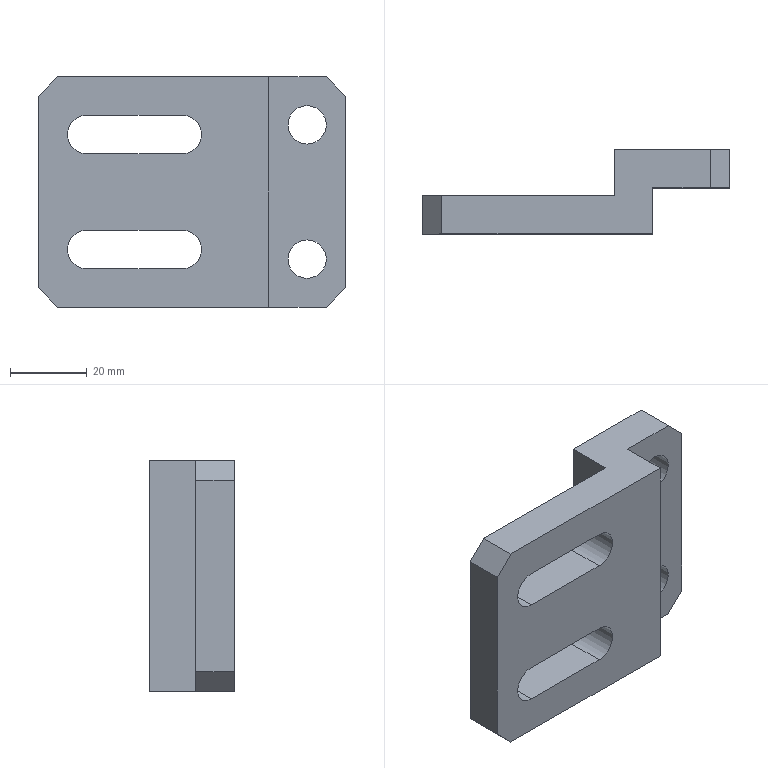Part | SolidWorks | features HoleWzd 2, Chamfer 1, Extrusion 1 | 1 solid | 26 faces | box 80 x 22 x 60 mm | volume 46558 mm3 | plane 18 | cylinder 8 | commonest cylinder face diameters 10 x8
STEP:
#1=CARTESIAN_POINT('',(10.,12.,-22.5));
#2=VERTEX_POINT('',#1);
#3=CARTESIAN_POINT('',(10.,12.,-12.5));
#4=VERTEX_POINT('',#3);
#5=CARTESIAN_POINT('',(10.,12.,-17.5));
#6=DIRECTION('',(0.,1.,0.));
#7=DIRECTION('',(0.,0.,1.));
#8=AXIS2_PLACEMENT_3D('',#5,#6,#7);
#9=CIRCLE('',#8,5.);
#10=EDGE_CURVE('',#2,#4,#9,.T.);
#11=ORIENTED_EDGE('',*,*,#10,.F.);
#12=CARTESIAN_POINT('',(10.,22.,-22.5));
#13=VERTEX_POINT('',#12);
#14=CARTESIAN_POINT('',(10.,22.,-22.5));
#15=DIRECTION('',(0.,1.,0.));
#16=VECTOR('',#15,1000.);
#17=LINE('',#14,#16);
#18=EDGE_CURVE('',#2,#13,#17,.T.);
#19=ORIENTED_EDGE('',*,*,#18,.T.);
#20=CARTESIAN_POINT('',(10.,22.,-12.5));
#21=VERTEX_POINT('',#20);
#22=CARTESIAN_POINT('',(10.,22.,-17.5));
#23=DIRECTION('',(0.,1.,0.));
#24=DIRECTION('',(0.,0.,1.));
#25=AXIS2_PLACEMENT_3D('',#22,#23,#24);
#26=CIRCLE('',#25,5.);
#27=EDGE_CURVE('',#13,#21,#26,.T.);
#28=ORIENTED_EDGE('',*,*,#27,.T.);
#29=CARTESIAN_POINT('',(10.,22.,-12.5));
#30=DIRECTION('',(0.,1.,0.));
#31=VECTOR('',#30,1000.);
#32=LINE('',#29,#31);
#33=EDGE_CURVE('',#4,#21,#32,.T.);
#34=ORIENTED_EDGE('',*,*,#33,.F.);
#35=EDGE_LOOP('',(#11,#19,#28,#34));
#36=FACE_OUTER_BOUND('',#35,.T.);
#37=CARTESIAN_POINT('',(10.,22.,-17.5));
#38=DIRECTION('',(0.,1.,0.));
#39=DIRECTION('',(0.,0.,1.));
#40=AXIS2_PLACEMENT_3D('',#37,#38,#39);
#41=CYLINDRICAL_SURFACE('',#40,5.);
#42=ADVANCED_FACE('',(#36),#41,.F.);
#43=CARTESIAN_POINT('',(10.,12.,12.5));
#44=VERTEX_POINT('',#43);
#45=CARTESIAN_POINT('',(10.,12.,22.5));
#46=VERTEX_POINT('',#45);
#47=CARTESIAN_POINT('',(10.,12.,17.5));
#48=DIRECTION('',(0.,1.,0.));
#49=DIRECTION('',(0.,0.,1.));
#50=AXIS2_PLACEMENT_3D('',#47,#48,#49);
#51=CIRCLE('',#50,5.);
#52=EDGE_CURVE('',#44,#46,#51,.T.);
#53=ORIENTED_EDGE('',*,*,#52,.F.);
#54=CARTESIAN_POINT('',(10.,22.,12.5));
#55=VERTEX_POINT('',#54);
#56=CARTESIAN_POINT('',(10.,22.,12.5));
#57=DIRECTION('',(0.,1.,0.));
#58=VECTOR('',#57,1000.);
#59=LINE('',#56,#58);
#60=EDGE_CURVE('',#44,#55,#59,.T.);
#61=ORIENTED_EDGE('',*,*,#60,.T.);
#62=CARTESIAN_POINT('',(10.,22.,22.5));
#63=VERTEX_POINT('',#62);
#64=CARTESIAN_POINT('',(10.,22.,17.5));
#65=DIRECTION('',(0.,1.,0.));
#66=DIRECTION('',(0.,0.,1.));
#67=AXIS2_PLACEMENT_3D('',#64,#65,#66);
#68=CIRCLE('',#67,5.);
#69=EDGE_CURVE('',#55,#63,#68,.T.);
#70=ORIENTED_EDGE('',*,*,#69,.T.);
#71=CARTESIAN_POINT('',(10.,22.,22.5));
#72=DIRECTION('',(0.,1.,0.));
#73=VECTOR('',#72,1000.);
#74=LINE('',#71,#73);
#75=EDGE_CURVE('',#46,#63,#74,.T.);
#76=ORIENTED_EDGE('',*,*,#75,.F.);
#77=EDGE_LOOP('',(#53,#61,#70,#76));
#78=FACE_OUTER_BOUND('',#77,.T.);
#79=CARTESIAN_POINT('',(10.,22.,17.5));
#80=DIRECTION('',(0.,1.,0.));
#81=DIRECTION('',(0.,0.,1.));
#82=AXIS2_PLACEMENT_3D('',#79,#80,#81);
#83=CYLINDRICAL_SURFACE('',#82,5.);
#84=ADVANCED_FACE('',(#78),#83,.F.);
#85=CARTESIAN_POINT('',(-10.,10.,-30.));
#86=VERTEX_POINT('',#85);
#87=CARTESIAN_POINT('',(-55.,10.,-30.));
#88=VERTEX_POINT('',#87);
#89=CARTESIAN_POINT('',(-10.,10.,-30.));
#90=DIRECTION('',(-1.,0.,0.));
#91=VECTOR('',#90,1000.);
#92=LINE('',#89,#91);
#93=EDGE_CURVE('',#86,#88,#92,.T.);
#94=ORIENTED_EDGE('',*,*,#93,.T.);
#95=CARTESIAN_POINT('',(-60.,10.,-25.));
#96=VERTEX_POINT('',#95);
#97=CARTESIAN_POINT('',(-60.,10.,-25.));
#98=DIRECTION('',(-0.7071,0.,0.7071));
#99=VECTOR('',#98,1000.);
#100=LINE('',#97,#99);
#101=EDGE_CURVE('',#88,#96,#100,.T.);
#102=ORIENTED_EDGE('',*,*,#101,.T.);
#103=CARTESIAN_POINT('',(-60.,10.,25.));
#104=VERTEX_POINT('',#103);
#105=CARTESIAN_POINT('',(-60.,10.,30.));
#106=DIRECTION('',(0.,0.,-1.));
#107=VECTOR('',#106,1000.);
#108=LINE('',#105,#107);
#109=EDGE_CURVE('',#104,#96,#108,.T.);
#110=ORIENTED_EDGE('',*,*,#109,.F.);
#111=CARTESIAN_POINT('',(-55.,10.,30.));
#112=VERTEX_POINT('',#111);
#113=CARTESIAN_POINT('',(-55.,10.,30.));
#114=DIRECTION('',(0.7071,0.,0.7071));
#115=VECTOR('',#114,1000.);
#116=LINE('',#113,#115);
#117=EDGE_CURVE('',#104,#112,#116,.T.);
#118=ORIENTED_EDGE('',*,*,#117,.T.);
#119=CARTESIAN_POINT('',(-10.,10.,30.));
#120=VERTEX_POINT('',#119);
#121=CARTESIAN_POINT('',(-10.,10.,30.));
#122=DIRECTION('',(-1.,0.,0.));
#123=VECTOR('',#122,1000.);
#124=LINE('',#121,#123);
#125=EDGE_CURVE('',#120,#112,#124,.T.);
#126=ORIENTED_EDGE('',*,*,#125,.F.);
#127=CARTESIAN_POINT('',(-10.,10.,30.));
#128=DIRECTION('',(0.,0.,-1.));
#129=VECTOR('',#128,1000.);
#130=LINE('',#127,#129);
#131=EDGE_CURVE('',#120,#86,#130,.T.);
#132=ORIENTED_EDGE('',*,*,#131,.T.);
#133=EDGE_LOOP('',(#94,#102,#110,#118,#126,#132));
#134=FACE_OUTER_BOUND('',#133,.T.);
#135=CARTESIAN_POINT('',(-47.5,10.,10.));
#136=VERTEX_POINT('',#135);
#137=CARTESIAN_POINT('',(-47.5,10.,20.));
#138=VERTEX_POINT('',#137);
#139=CARTESIAN_POINT('',(-47.5,10.,15.));
#140=DIRECTION('',(0.,1.,0.));
#141=DIRECTION('',(0.,0.,1.));
#142=AXIS2_PLACEMENT_3D('',#139,#140,#141);
#143=CIRCLE('',#142,5.);
#144=EDGE_CURVE('',#136,#138,#143,.T.);
#145=ORIENTED_EDGE('',*,*,#144,.F.);
#146=CARTESIAN_POINT('',(-22.5,10.,10.));
#147=VERTEX_POINT('',#146);
#148=CARTESIAN_POINT('',(-47.5,10.,10.));
#149=DIRECTION('',(1.,0.,0.));
#150=VECTOR('',#149,1000.);
#151=LINE('',#148,#150);
#152=EDGE_CURVE('',#136,#147,#151,.T.);
#153=ORIENTED_EDGE('',*,*,#152,.T.);
#154=CARTESIAN_POINT('',(-22.5,10.,20.));
#155=VERTEX_POINT('',#154);
#156=CARTESIAN_POINT('',(-22.5,10.,15.));
#157=DIRECTION('',(0.,1.,0.));
#158=DIRECTION('',(0.,0.,1.));
#159=AXIS2_PLACEMENT_3D('',#156,#157,#158);
#160=CIRCLE('',#159,5.);
#161=EDGE_CURVE('',#155,#147,#160,.T.);
#162=ORIENTED_EDGE('',*,*,#161,.F.);
#163=CARTESIAN_POINT('',(-47.5,10.,20.));
#164=DIRECTION('',(1.,0.,0.));
#165=VECTOR('',#164,1000.);
#166=LINE('',#163,#165);
#167=EDGE_CURVE('',#138,#155,#166,.T.);
#168=ORIENTED_EDGE('',*,*,#167,.F.);
#169=EDGE_LOOP('',(#145,#153,#162,#168));
#170=FACE_BOUND('',#169,.T.);
#171=CARTESIAN_POINT('',(-47.5,10.,-10.));
#172=VERTEX_POINT('',#171);
#173=CARTESIAN_POINT('',(-22.5,10.,-10.));
#174=VERTEX_POINT('',#173);
#175=CARTESIAN_POINT('',(-47.5,10.,-10.));
#176=DIRECTION('',(1.,0.,0.));
#177=VECTOR('',#176,1000.);
#178=LINE('',#175,#177);
#179=EDGE_CURVE('',#172,#174,#178,.T.);
#180=ORIENTED_EDGE('',*,*,#179,.F.);
#181=CARTESIAN_POINT('',(-47.5,10.,-20.));
#182=VERTEX_POINT('',#181);
#183=CARTESIAN_POINT('',(-47.5,10.,-15.));
#184=DIRECTION('',(0.,1.,0.));
#185=DIRECTION('',(0.,0.,1.));
#186=AXIS2_PLACEMENT_3D('',#183,#184,#185);
#187=CIRCLE('',#186,5.);
#188=EDGE_CURVE('',#182,#172,#187,.T.);
#189=ORIENTED_EDGE('',*,*,#188,.F.);
#190=CARTESIAN_POINT('',(-22.5,10.,-20.));
#191=VERTEX_POINT('',#190);
#192=CARTESIAN_POINT('',(-47.5,10.,-20.));
#193=DIRECTION('',(1.,0.,0.));
#194=VECTOR('',#193,1000.);
#195=LINE('',#192,#194);
#196=EDGE_CURVE('',#182,#191,#195,.T.);
#197=ORIENTED_EDGE('',*,*,#196,.T.);
#198=CARTESIAN_POINT('',(-22.5,10.,-15.));
#199=DIRECTION('',(0.,1.,0.));
#200=DIRECTION('',(0.,0.,1.));
#201=AXIS2_PLACEMENT_3D('',#198,#199,#200);
#202=CIRCLE('',#201,5.);
#203=EDGE_CURVE('',#174,#191,#202,.T.);
#204=ORIENTED_EDGE('',*,*,#203,.F.);
#205=EDGE_LOOP('',(#180,#189,#197,#204));
#206=FACE_BOUND('',#205,.T.);
#207=CARTESIAN_POINT('',(-10.,10.,30.));
#208=DIRECTION('',(0.,-1.,0.));
#209=DIRECTION('',(1.,0.,0.));
#210=AXIS2_PLACEMENT_3D('',#207,#208,#209);
#211=PLANE('',#210);
#212=ADVANCED_FACE('',(#134,#170,#206),#211,.F.);
#213=CARTESIAN_POINT('',(-47.5,0.,-10.));
#214=VERTEX_POINT('',#213);
#215=CARTESIAN_POINT('',(-22.5,0.,-10.));
#216=VERTEX_POINT('',#215);
#217=CARTESIAN_POINT('',(-47.5,0.,-10.));
#218=DIRECTION('',(1.,0.,0.));
#219=VECTOR('',#218,1000.);
#220=LINE('',#217,#219);
#221=EDGE_CURVE('',#214,#216,#220,.T.);
#222=ORIENTED_EDGE('',*,*,#221,.T.);
#223=CARTESIAN_POINT('',(-22.5,0.,-20.));
#224=VERTEX_POINT('',#223);
#225=CARTESIAN_POINT('',(-22.5,0.,-15.));
#226=DIRECTION('',(0.,1.,0.));
#227=DIRECTION('',(0.,0.,1.));
#228=AXIS2_PLACEMENT_3D('',#225,#226,#227);
#229=CIRCLE('',#228,5.);
#230=EDGE_CURVE('',#216,#224,#229,.T.);
#231=ORIENTED_EDGE('',*,*,#230,.T.);
#232=CARTESIAN_POINT('',(-47.5,0.,-20.));
#233=VERTEX_POINT('',#232);
#234=CARTESIAN_POINT('',(-47.5,0.,-20.));
#235=DIRECTION('',(1.,0.,0.));
#236=VECTOR('',#235,1000.);
#237=LINE('',#234,#236);
#238=EDGE_CURVE('',#233,#224,#237,.T.);
#239=ORIENTED_EDGE('',*,*,#238,.F.);
#240=CARTESIAN_POINT('',(-47.5,0.,-15.));
#241=DIRECTION('',(0.,1.,0.));
#242=DIRECTION('',(0.,0.,1.));
#243=AXIS2_PLACEMENT_3D('',#240,#241,#242);
#244=CIRCLE('',#243,5.);
#245=EDGE_CURVE('',#233,#214,#244,.T.);
#246=ORIENTED_EDGE('',*,*,#245,.T.);
#247=EDGE_LOOP('',(#222,#231,#239,#246));
#248=FACE_BOUND('',#247,.T.);
#249=CARTESIAN_POINT('',(-60.,0.,25.));
#250=VERTEX_POINT('',#249);
#251=CARTESIAN_POINT('',(-60.,0.,-25.));
#252=VERTEX_POINT('',#251);
#253=CARTESIAN_POINT('',(-60.,0.,30.));
#254=DIRECTION('',(0.,0.,-1.));
#255=VECTOR('',#254,1000.);
#256=LINE('',#253,#255);
#257=EDGE_CURVE('',#250,#252,#256,.T.);
#258=ORIENTED_EDGE('',*,*,#257,.T.);
#259=CARTESIAN_POINT('',(-55.,0.,-30.));
#260=VERTEX_POINT('',#259);
#261=CARTESIAN_POINT('',(-60.,0.,-25.));
#262=DIRECTION('',(0.7071,0.,-0.7071));
#263=VECTOR('',#262,1000.);
#264=LINE('',#261,#263);
#265=EDGE_CURVE('',#252,#260,#264,.T.);
#266=ORIENTED_EDGE('',*,*,#265,.T.);
#267=CARTESIAN_POINT('',(0.,0.,-30.));
#268=VERTEX_POINT('',#267);
#269=CARTESIAN_POINT('',(0.,0.,-30.));
#270=DIRECTION('',(1.,0.,0.));
#271=VECTOR('',#270,1000.);
#272=LINE('',#269,#271);
#273=EDGE_CURVE('',#260,#268,#272,.T.);
#274=ORIENTED_EDGE('',*,*,#273,.T.);
#275=CARTESIAN_POINT('',(0.,0.,30.));
#276=VERTEX_POINT('',#275);
#277=CARTESIAN_POINT('',(0.,0.,30.));
#278=DIRECTION('',(0.,0.,-1.));
#279=VECTOR('',#278,1000.);
#280=LINE('',#277,#279);
#281=EDGE_CURVE('',#276,#268,#280,.T.);
#282=ORIENTED_EDGE('',*,*,#281,.F.);
#283=CARTESIAN_POINT('',(-55.,0.,30.));
#284=VERTEX_POINT('',#283);
#285=CARTESIAN_POINT('',(0.,0.,30.));
#286=DIRECTION('',(1.,0.,0.));
#287=VECTOR('',#286,1000.);
#288=LINE('',#285,#287);
#289=EDGE_CURVE('',#284,#276,#288,.T.);
#290=ORIENTED_EDGE('',*,*,#289,.F.);
#291=CARTESIAN_POINT('',(-55.,0.,30.));
#292=DIRECTION('',(-0.7071,0.,-0.7071));
#293=VECTOR('',#292,1000.);
#294=LINE('',#291,#293);
#295=EDGE_CURVE('',#284,#250,#294,.T.);
#296=ORIENTED_EDGE('',*,*,#295,.T.);
#297=EDGE_LOOP('',(#258,#266,#274,#282,#290,#296));
#298=FACE_OUTER_BOUND('',#297,.T.);
#299=CARTESIAN_POINT('',(-47.5,0.,10.));
#300=VERTEX_POINT('',#299);
#301=CARTESIAN_POINT('',(-22.5,0.,10.));
#302=VERTEX_POINT('',#301);
#303=CARTESIAN_POINT('',(-47.5,0.,10.));
#304=DIRECTION('',(1.,0.,0.));
#305=VECTOR('',#304,1000.);
#306=LINE('',#303,#305);
#307=EDGE_CURVE('',#300,#302,#306,.T.);
#308=ORIENTED_EDGE('',*,*,#307,.F.);
#309=CARTESIAN_POINT('',(-47.5,0.,20.));
#310=VERTEX_POINT('',#309);
#311=CARTESIAN_POINT('',(-47.5,0.,15.));
#312=DIRECTION('',(0.,1.,0.));
#313=DIRECTION('',(0.,0.,1.));
#314=AXIS2_PLACEMENT_3D('',#311,#312,#313);
#315=CIRCLE('',#314,5.);
#316=EDGE_CURVE('',#300,#310,#315,.T.);
#317=ORIENTED_EDGE('',*,*,#316,.T.);
#318=CARTESIAN_POINT('',(-22.5,0.,20.));
#319=VERTEX_POINT('',#318);
#320=CARTESIAN_POINT('',(-47.5,0.,20.));
#321=DIRECTION('',(1.,0.,0.));
#322=VECTOR('',#321,1000.);
#323=LINE('',#320,#322);
#324=EDGE_CURVE('',#310,#319,#323,.T.);
#325=ORIENTED_EDGE('',*,*,#324,.T.);
#326=CARTESIAN_POINT('',(-22.5,0.,15.));
#327=DIRECTION('',(0.,1.,0.));
#328=DIRECTION('',(0.,0.,1.));
#329=AXIS2_PLACEMENT_3D('',#326,#327,#328);
#330=CIRCLE('',#329,5.);
#331=EDGE_CURVE('',#319,#302,#330,.T.);
#332=ORIENTED_EDGE('',*,*,#331,.T.);
#333=EDGE_LOOP('',(#308,#317,#325,#332));
#334=FACE_BOUND('',#333,.T.);
#335=CARTESIAN_POINT('',(0.,0.,30.));
#336=DIRECTION('',(0.,1.,0.));
#337=DIRECTION('',(-1.,0.,0.));
#338=AXIS2_PLACEMENT_3D('',#335,#336,#337);
#339=PLANE('',#338);
#340=ADVANCED_FACE('',(#248,#298,#334),#339,.F.);
#341=CARTESIAN_POINT('',(0.,12.,-30.));
#342=VERTEX_POINT('',#341);
#343=CARTESIAN_POINT('',(0.,0.,-30.));
#344=DIRECTION('',(0.,1.,0.));
#345=VECTOR('',#344,1000.);
#346=LINE('',#343,#345);
#347=EDGE_CURVE('',#268,#342,#346,.T.);
#348=ORIENTED_EDGE('',*,*,#347,.T.);
#349=CARTESIAN_POINT('',(0.,12.,30.));
#350=VERTEX_POINT('',#349);
#351=CARTESIAN_POINT('',(0.,12.,30.));
#352=DIRECTION('',(0.,0.,-1.));
#353=VECTOR('',#352,1000.);
#354=LINE('',#351,#353);
#355=EDGE_CURVE('',#350,#342,#354,.T.);
#356=ORIENTED_EDGE('',*,*,#355,.F.);
#357=CARTESIAN_POINT('',(0.,0.,30.));
#358=DIRECTION('',(0.,1.,0.));
#359=VECTOR('',#358,1000.);
#360=LINE('',#357,#359);
#361=EDGE_CURVE('',#276,#350,#360,.T.);
#362=ORIENTED_EDGE('',*,*,#361,.F.);
#363=ORIENTED_EDGE('',*,*,#281,.T.);
#364=EDGE_LOOP('',(#348,#356,#362,#363));
#365=FACE_OUTER_BOUND('',#364,.T.);
#366=CARTESIAN_POINT('',(0.,0.,30.));
#367=DIRECTION('',(-1.,0.,0.));
#368=DIRECTION('',(0.,0.,1.));
#369=AXIS2_PLACEMENT_3D('',#366,#367,#368);
#370=PLANE('',#369);
#371=ADVANCED_FACE('',(#365),#370,.F.);
#372=CARTESIAN_POINT('',(10.,12.,-17.5));
#373=DIRECTION('',(0.,1.,0.));
#374=DIRECTION('',(0.,0.,1.));
#375=AXIS2_PLACEMENT_3D('',#372,#373,#374);
#376=CIRCLE('',#375,5.);
#377=EDGE_CURVE('',#4,#2,#376,.T.);
#378=ORIENTED_EDGE('',*,*,#377,.T.);
#379=ORIENTED_EDGE('',*,*,#10,.T.);
#380=EDGE_LOOP('',(#378,#379));
#381=FACE_BOUND('',#380,.T.);
#382=CARTESIAN_POINT('',(10.,12.,17.5));
#383=DIRECTION('',(0.,1.,0.));
#384=DIRECTION('',(0.,0.,1.));
#385=AXIS2_PLACEMENT_3D('',#382,#383,#384);
#386=CIRCLE('',#385,5.);
#387=EDGE_CURVE('',#46,#44,#386,.T.);
#388=ORIENTED_EDGE('',*,*,#387,.T.);
#389=ORIENTED_EDGE('',*,*,#52,.T.);
#390=EDGE_LOOP('',(#388,#389));
#391=FACE_BOUND('',#390,.T.);
#392=CARTESIAN_POINT('',(15.,12.,-30.));
#393=VERTEX_POINT('',#392);
#394=CARTESIAN_POINT('',(0.,12.,-30.));
#395=DIRECTION('',(1.,0.,0.));
#396=VECTOR('',#395,1000.);
#397=LINE('',#394,#396);
#398=EDGE_CURVE('',#342,#393,#397,.T.);
#399=ORIENTED_EDGE('',*,*,#398,.T.);
#400=CARTESIAN_POINT('',(20.,12.,-25.));
#401=VERTEX_POINT('',#400);
#402=CARTESIAN_POINT('',(20.,12.,-25.));
#403=DIRECTION('',(0.7071,0.,0.7071));
#404=VECTOR('',#403,1000.);
#405=LINE('',#402,#404);
#406=EDGE_CURVE('',#393,#401,#405,.T.);
#407=ORIENTED_EDGE('',*,*,#406,.T.);
#408=CARTESIAN_POINT('',(20.,12.,25.));
#409=VERTEX_POINT('',#408);
#410=CARTESIAN_POINT('',(20.,12.,30.));
#411=DIRECTION('',(0.,0.,-1.));
#412=VECTOR('',#411,1000.);
#413=LINE('',#410,#412);
#414=EDGE_CURVE('',#409,#401,#413,.T.);
#415=ORIENTED_EDGE('',*,*,#414,.F.);
#416=CARTESIAN_POINT('',(15.,12.,30.));
#417=VERTEX_POINT('',#416);
#418=CARTESIAN_POINT('',(15.,12.,30.));
#419=DIRECTION('',(-0.7071,0.,0.7071));
#420=VECTOR('',#419,1000.);
#421=LINE('',#418,#420);
#422=EDGE_CURVE('',#409,#417,#421,.T.);
#423=ORIENTED_EDGE('',*,*,#422,.T.);
#424=CARTESIAN_POINT('',(0.,12.,30.));
#425=DIRECTION('',(1.,0.,0.));
#426=VECTOR('',#425,1000.);
#427=LINE('',#424,#426);
#428=EDGE_CURVE('',#350,#417,#427,.T.);
#429=ORIENTED_EDGE('',*,*,#428,.F.);
#430=ORIENTED_EDGE('',*,*,#355,.T.);
#431=EDGE_LOOP('',(#399,#407,#415,#423,#429,#430));
#432=FACE_OUTER_BOUND('',#431,.T.);
#433=CARTESIAN_POINT('',(0.,12.,30.));
#434=DIRECTION('',(0.,1.,0.));
#435=DIRECTION('',(0.,0.,1.));
#436=AXIS2_PLACEMENT_3D('',#433,#434,#435);
#437=PLANE('',#436);
#438=ADVANCED_FACE('',(#381,#391,#432),#437,.F.);
#439=ORIENTED_EDGE('',*,*,#414,.T.);
#440=CARTESIAN_POINT('',(20.,22.,-25.));
#441=VERTEX_POINT('',#440);
#442=CARTESIAN_POINT('',(20.,22.,-25.));
#443=DIRECTION('',(0.,1.,0.));
#444=VECTOR('',#443,1000.);
#445=LINE('',#442,#444);
#446=EDGE_CURVE('',#401,#441,#445,.T.);
#447=ORIENTED_EDGE('',*,*,#446,.T.);
#448=CARTESIAN_POINT('',(20.,22.,25.));
#449=VERTEX_POINT('',#448);
#450=CARTESIAN_POINT('',(20.,22.,30.));
#451=DIRECTION('',(0.,0.,-1.));
#452=VECTOR('',#451,1000.);
#453=LINE('',#450,#452);
#454=EDGE_CURVE('',#449,#441,#453,.T.);
#455=ORIENTED_EDGE('',*,*,#454,.F.);
#456=CARTESIAN_POINT('',(20.,12.,25.));
#457=DIRECTION('',(0.,-1.,0.));
#458=VECTOR('',#457,1000.);
#459=LINE('',#456,#458);
#460=EDGE_CURVE('',#449,#409,#459,.T.);
#461=ORIENTED_EDGE('',*,*,#460,.T.);
#462=EDGE_LOOP('',(#439,#447,#455,#461));
#463=FACE_OUTER_BOUND('',#462,.T.);
#464=CARTESIAN_POINT('',(20.,22.,30.));
#465=DIRECTION('',(-1.,0.,0.));
#466=DIRECTION('',(0.,0.,1.));
#467=AXIS2_PLACEMENT_3D('',#464,#465,#466);
#468=PLANE('',#467);
#469=ADVANCED_FACE('',(#463),#468,.F.);
#470=CARTESIAN_POINT('',(10.,22.,-17.5));
#471=DIRECTION('',(0.,1.,0.));
#472=DIRECTION('',(0.,0.,1.));
#473=AXIS2_PLACEMENT_3D('',#470,#471,#472);
#474=CIRCLE('',#473,5.);
#475=EDGE_CURVE('',#21,#13,#474,.T.);
#476=ORIENTED_EDGE('',*,*,#475,.F.);
#477=ORIENTED_EDGE('',*,*,#27,.F.);
#478=EDGE_LOOP('',(#476,#477));
#479=FACE_BOUND('',#478,.T.);
#480=CARTESIAN_POINT('',(10.,22.,17.5));
#481=DIRECTION('',(0.,1.,0.));
#482=DIRECTION('',(0.,0.,1.));
#483=AXIS2_PLACEMENT_3D('',#480,#481,#482);
#484=CIRCLE('',#483,5.);
#485=EDGE_CURVE('',#63,#55,#484,.T.);
#486=ORIENTED_EDGE('',*,*,#485,.F.);
#487=ORIENTED_EDGE('',*,*,#69,.F.);
#488=EDGE_LOOP('',(#486,#487));
#489=FACE_BOUND('',#488,.T.);
#490=ORIENTED_EDGE('',*,*,#454,.T.);
#491=CARTESIAN_POINT('',(15.,22.,-30.));
#492=VERTEX_POINT('',#491);
#493=CARTESIAN_POINT('',(20.,22.,-25.));
#494=DIRECTION('',(-0.7071,0.,-0.7071));
#495=VECTOR('',#494,1000.);
#496=LINE('',#493,#495);
#497=EDGE_CURVE('',#441,#492,#496,.T.);
#498=ORIENTED_EDGE('',*,*,#497,.T.);
#499=CARTESIAN_POINT('',(-10.,22.,-30.));
#500=VERTEX_POINT('',#499);
#501=CARTESIAN_POINT('',(-10.,22.,-30.));
#502=DIRECTION('',(-1.,0.,0.));
#503=VECTOR('',#502,1000.);
#504=LINE('',#501,#503);
#505=EDGE_CURVE('',#492,#500,#504,.T.);
#506=ORIENTED_EDGE('',*,*,#505,.T.);
#507=CARTESIAN_POINT('',(-10.,22.,30.));
#508=VERTEX_POINT('',#507);
#509=CARTESIAN_POINT('',(-10.,22.,30.));
#510=DIRECTION('',(0.,0.,-1.));
#511=VECTOR('',#510,1000.);
#512=LINE('',#509,#511);
#513=EDGE_CURVE('',#508,#500,#512,.T.);
#514=ORIENTED_EDGE('',*,*,#513,.F.);
#515=CARTESIAN_POINT('',(15.,22.,30.));
#516=VERTEX_POINT('',#515);
#517=CARTESIAN_POINT('',(-10.,22.,30.));
#518=DIRECTION('',(-1.,0.,0.));
#519=VECTOR('',#518,1000.);
#520=LINE('',#517,#519);
#521=EDGE_CURVE('',#516,#508,#520,.T.);
#522=ORIENTED_EDGE('',*,*,#521,.F.);
#523=CARTESIAN_POINT('',(15.,22.,30.));
#524=DIRECTION('',(0.7071,0.,-0.7071));
#525=VECTOR('',#524,1000.);
#526=LINE('',#523,#525);
#527=EDGE_CURVE('',#516,#449,#526,.T.);
#528=ORIENTED_EDGE('',*,*,#527,.T.);
#529=EDGE_LOOP('',(#490,#498,#506,#514,#522,#528));
#530=FACE_OUTER_BOUND('',#529,.T.);
#531=CARTESIAN_POINT('',(-10.,22.,30.));
#532=DIRECTION('',(0.,-1.,0.));
#533=DIRECTION('',(0.,0.,-1.));
#534=AXIS2_PLACEMENT_3D('',#531,#532,#533);
#535=PLANE('',#534);
#536=ADVANCED_FACE('',(#479,#489,#530),#535,.F.);
#537=CARTESIAN_POINT('',(-10.,10.,-30.));
#538=DIRECTION('',(0.,-1.,0.));
#539=VECTOR('',#538,1000.);
#540=LINE('',#537,#539);
#541=EDGE_CURVE('',#500,#86,#540,.T.);
#542=ORIENTED_EDGE('',*,*,#541,.T.);
#543=ORIENTED_EDGE('',*,*,#131,.F.);
#544=CARTESIAN_POINT('',(-10.,10.,30.));
#545=DIRECTION('',(0.,-1.,0.));
#546=VECTOR('',#545,1000.);
#547=LINE('',#544,#546);
#548=EDGE_CURVE('',#508,#120,#547,.T.);
#549=ORIENTED_EDGE('',*,*,#548,.F.);
#550=ORIENTED_EDGE('',*,*,#513,.T.);
#551=EDGE_LOOP('',(#542,#543,#549,#550));
#552=FACE_OUTER_BOUND('',#551,.T.);
#553=CARTESIAN_POINT('',(-10.,10.,30.));
#554=DIRECTION('',(1.,0.,0.));
#555=DIRECTION('',(0.,0.,-1.));
#556=AXIS2_PLACEMENT_3D('',#553,#554,#555);
#557=PLANE('',#556);
#558=ADVANCED_FACE('',(#552),#557,.F.);
#559=ORIENTED_EDGE('',*,*,#109,.T.);
#560=CARTESIAN_POINT('',(-60.,10.,-25.));
#561=DIRECTION('',(0.,-1.,0.));
#562=VECTOR('',#561,1000.);
#563=LINE('',#560,#562);
#564=EDGE_CURVE('',#96,#252,#563,.T.);
#565=ORIENTED_EDGE('',*,*,#564,.T.);
#566=ORIENTED_EDGE('',*,*,#257,.F.);
#567=CARTESIAN_POINT('',(-60.,10.,25.));
#568=DIRECTION('',(0.,1.,0.));
#569=VECTOR('',#568,1000.);
#570=LINE('',#567,#569);
#571=EDGE_CURVE('',#250,#104,#570,.T.);
#572=ORIENTED_EDGE('',*,*,#571,.T.);
#573=EDGE_LOOP('',(#559,#565,#566,#572));
#574=FACE_OUTER_BOUND('',#573,.T.);
#575=CARTESIAN_POINT('',(-60.,10.,30.));
#576=DIRECTION('',(1.,0.,0.));
#577=DIRECTION('',(0.,0.,-1.));
#578=AXIS2_PLACEMENT_3D('',#575,#576,#577);
#579=PLANE('',#578);
#580=ADVANCED_FACE('',(#574),#579,.F.);
#581=ORIENTED_EDGE('',*,*,#125,.T.);
#582=CARTESIAN_POINT('',(-55.,0.,30.));
#583=DIRECTION('',(0.,-1.,0.));
#584=VECTOR('',#583,1000.);
#585=LINE('',#582,#584);
#586=EDGE_CURVE('',#112,#284,#585,.T.);
#587=ORIENTED_EDGE('',*,*,#586,.T.);
#588=ORIENTED_EDGE('',*,*,#289,.T.);
#589=ORIENTED_EDGE('',*,*,#361,.T.);
#590=ORIENTED_EDGE('',*,*,#428,.T.);
#591=CARTESIAN_POINT('',(15.,22.,30.));
#592=DIRECTION('',(0.,1.,0.));
#593=VECTOR('',#592,1000.);
#594=LINE('',#591,#593);
#595=EDGE_CURVE('',#417,#516,#594,.T.);
#596=ORIENTED_EDGE('',*,*,#595,.T.);
#597=ORIENTED_EDGE('',*,*,#521,.T.);
#598=ORIENTED_EDGE('',*,*,#548,.T.);
#599=EDGE_LOOP('',(#581,#587,#588,#589,#590,#596,#597,#598));
#600=FACE_OUTER_BOUND('',#599,.T.);
#601=CARTESIAN_POINT('',(0.,0.,30.));
#602=DIRECTION('',(0.,0.,1.));
#603=DIRECTION('',(1.,0.,0.));
#604=AXIS2_PLACEMENT_3D('',#601,#602,#603);
#605=PLANE('',#604);
#606=ADVANCED_FACE('',(#600),#605,.T.);
#607=ORIENTED_EDGE('',*,*,#273,.F.);
#608=CARTESIAN_POINT('',(-55.,0.,-30.));
#609=DIRECTION('',(0.,1.,0.));
#610=VECTOR('',#609,1000.);
#611=LINE('',#608,#610);
#612=EDGE_CURVE('',#260,#88,#611,.T.);
#613=ORIENTED_EDGE('',*,*,#612,.T.);
#614=ORIENTED_EDGE('',*,*,#93,.F.);
#615=ORIENTED_EDGE('',*,*,#541,.F.);
#616=ORIENTED_EDGE('',*,*,#505,.F.);
#617=CARTESIAN_POINT('',(15.,0.,-30.));
#618=DIRECTION('',(0.,-1.,0.));
#619=VECTOR('',#618,1000.);
#620=LINE('',#617,#619);
#621=EDGE_CURVE('',#492,#393,#620,.T.);
#622=ORIENTED_EDGE('',*,*,#621,.T.);
#623=ORIENTED_EDGE('',*,*,#398,.F.);
#624=ORIENTED_EDGE('',*,*,#347,.F.);
#625=EDGE_LOOP('',(#607,#613,#614,#615,#616,#622,#623,#624));
#626=FACE_OUTER_BOUND('',#625,.T.);
#627=CARTESIAN_POINT('',(0.,0.,-30.));
#628=DIRECTION('',(0.,0.,1.));
#629=DIRECTION('',(1.,0.,0.));
#630=AXIS2_PLACEMENT_3D('',#627,#628,#629);
#631=PLANE('',#630);
#632=ADVANCED_FACE('',(#626),#631,.F.);
#633=ORIENTED_EDGE('',*,*,#60,.F.);
#634=ORIENTED_EDGE('',*,*,#387,.F.);
#635=ORIENTED_EDGE('',*,*,#75,.T.);
#636=ORIENTED_EDGE('',*,*,#485,.T.);
#637=EDGE_LOOP('',(#633,#634,#635,#636));
#638=FACE_OUTER_BOUND('',#637,.T.);
#639=CARTESIAN_POINT('',(10.,22.,17.5));
#640=DIRECTION('',(0.,1.,0.));
#641=DIRECTION('',(0.,0.,1.));
#642=AXIS2_PLACEMENT_3D('',#639,#640,#641);
#643=CYLINDRICAL_SURFACE('',#642,5.);
#644=ADVANCED_FACE('',(#638),#643,.F.);
#645=ORIENTED_EDGE('',*,*,#18,.F.);
#646=ORIENTED_EDGE('',*,*,#377,.F.);
#647=ORIENTED_EDGE('',*,*,#33,.T.);
#648=ORIENTED_EDGE('',*,*,#475,.T.);
#649=EDGE_LOOP('',(#645,#646,#647,#648));
#650=FACE_OUTER_BOUND('',#649,.T.);
#651=CARTESIAN_POINT('',(10.,22.,-17.5));
#652=DIRECTION('',(0.,1.,0.));
#653=DIRECTION('',(0.,0.,1.));
#654=AXIS2_PLACEMENT_3D('',#651,#652,#653);
#655=CYLINDRICAL_SURFACE('',#654,5.);
#656=ADVANCED_FACE('',(#650),#655,.F.);
#657=ORIENTED_EDGE('',*,*,#331,.F.);
#658=CARTESIAN_POINT('',(-22.5,10.,20.));
#659=DIRECTION('',(0.,-1.,0.));
#660=VECTOR('',#659,1000.);
#661=LINE('',#658,#660);
#662=EDGE_CURVE('',#155,#319,#661,.T.);
#663=ORIENTED_EDGE('',*,*,#662,.F.);
#664=ORIENTED_EDGE('',*,*,#161,.T.);
#665=CARTESIAN_POINT('',(-22.5,10.,10.));
#666=DIRECTION('',(0.,1.,0.));
#667=VECTOR('',#666,1000.);
#668=LINE('',#665,#667);
#669=EDGE_CURVE('',#302,#147,#668,.T.);
#670=ORIENTED_EDGE('',*,*,#669,.F.);
#671=EDGE_LOOP('',(#657,#663,#664,#670));
#672=FACE_OUTER_BOUND('',#671,.T.);
#673=CARTESIAN_POINT('',(-22.5,10.,15.));
#674=DIRECTION('',(0.,1.,0.));
#675=DIRECTION('',(0.,0.,1.));
#676=AXIS2_PLACEMENT_3D('',#673,#674,#675);
#677=CYLINDRICAL_SURFACE('',#676,5.);
#678=ADVANCED_FACE('',(#672),#677,.F.);
#679=ORIENTED_EDGE('',*,*,#144,.T.);
#680=CARTESIAN_POINT('',(-47.5,10.,20.));
#681=DIRECTION('',(0.,1.,0.));
#682=VECTOR('',#681,1000.);
#683=LINE('',#680,#682);
#684=EDGE_CURVE('',#310,#138,#683,.T.);
#685=ORIENTED_EDGE('',*,*,#684,.F.);
#686=ORIENTED_EDGE('',*,*,#316,.F.);
#687=CARTESIAN_POINT('',(-47.5,10.,10.));
#688=DIRECTION('',(0.,-1.,0.));
#689=VECTOR('',#688,1000.);
#690=LINE('',#687,#689);
#691=EDGE_CURVE('',#136,#300,#690,.T.);
#692=ORIENTED_EDGE('',*,*,#691,.F.);
#693=EDGE_LOOP('',(#679,#685,#686,#692));
#694=FACE_OUTER_BOUND('',#693,.T.);
#695=CARTESIAN_POINT('',(-47.5,10.,15.));
#696=DIRECTION('',(0.,1.,0.));
#697=DIRECTION('',(0.,0.,1.));
#698=AXIS2_PLACEMENT_3D('',#695,#696,#697);
#699=CYLINDRICAL_SURFACE('',#698,5.);
#700=ADVANCED_FACE('',(#694),#699,.F.);
#701=ORIENTED_EDGE('',*,*,#669,.T.);
#702=ORIENTED_EDGE('',*,*,#152,.F.);
#703=ORIENTED_EDGE('',*,*,#691,.T.);
#704=ORIENTED_EDGE('',*,*,#307,.T.);
#705=EDGE_LOOP('',(#701,#702,#703,#704));
#706=FACE_OUTER_BOUND('',#705,.T.);
#707=CARTESIAN_POINT('',(-47.5,10.,10.));
#708=DIRECTION('',(0.,0.,-1.));
#709=DIRECTION('',(-1.,0.,0.));
#710=AXIS2_PLACEMENT_3D('',#707,#708,#709);
#711=PLANE('',#710);
#712=ADVANCED_FACE('',(#706),#711,.F.);
#713=ORIENTED_EDGE('',*,*,#662,.T.);
#714=ORIENTED_EDGE('',*,*,#324,.F.);
#715=ORIENTED_EDGE('',*,*,#684,.T.);
#716=ORIENTED_EDGE('',*,*,#167,.T.);
#717=EDGE_LOOP('',(#713,#714,#715,#716));
#718=FACE_OUTER_BOUND('',#717,.T.);
#719=CARTESIAN_POINT('',(-47.5,10.,20.));
#720=DIRECTION('',(0.,0.,1.));
#721=DIRECTION('',(1.,0.,0.));
#722=AXIS2_PLACEMENT_3D('',#719,#720,#721);
#723=PLANE('',#722);
#724=ADVANCED_FACE('',(#718),#723,.F.);
#725=ORIENTED_EDGE('',*,*,#230,.F.);
#726=CARTESIAN_POINT('',(-22.5,10.,-10.));
#727=DIRECTION('',(0.,-1.,0.));
#728=VECTOR('',#727,1000.);
#729=LINE('',#726,#728);
#730=EDGE_CURVE('',#174,#216,#729,.T.);
#731=ORIENTED_EDGE('',*,*,#730,.F.);
#732=ORIENTED_EDGE('',*,*,#203,.T.);
#733=CARTESIAN_POINT('',(-22.5,10.,-20.));
#734=DIRECTION('',(0.,1.,0.));
#735=VECTOR('',#734,1000.);
#736=LINE('',#733,#735);
#737=EDGE_CURVE('',#224,#191,#736,.T.);
#738=ORIENTED_EDGE('',*,*,#737,.F.);
#739=EDGE_LOOP('',(#725,#731,#732,#738));
#740=FACE_OUTER_BOUND('',#739,.T.);
#741=CARTESIAN_POINT('',(-22.5,10.,-15.));
#742=DIRECTION('',(0.,1.,0.));
#743=DIRECTION('',(0.,0.,1.));
#744=AXIS2_PLACEMENT_3D('',#741,#742,#743);
#745=CYLINDRICAL_SURFACE('',#744,5.);
#746=ADVANCED_FACE('',(#740),#745,.F.);
#747=ORIENTED_EDGE('',*,*,#188,.T.);
#748=CARTESIAN_POINT('',(-47.5,10.,-10.));
#749=DIRECTION('',(0.,1.,0.));
#750=VECTOR('',#749,1000.);
#751=LINE('',#748,#750);
#752=EDGE_CURVE('',#214,#172,#751,.T.);
#753=ORIENTED_EDGE('',*,*,#752,.F.);
#754=ORIENTED_EDGE('',*,*,#245,.F.);
#755=CARTESIAN_POINT('',(-47.5,10.,-20.));
#756=DIRECTION('',(0.,-1.,0.));
#757=VECTOR('',#756,1000.);
#758=LINE('',#755,#757);
#759=EDGE_CURVE('',#182,#233,#758,.T.);
#760=ORIENTED_EDGE('',*,*,#759,.F.);
#761=EDGE_LOOP('',(#747,#753,#754,#760));
#762=FACE_OUTER_BOUND('',#761,.T.);
#763=CARTESIAN_POINT('',(-47.5,10.,-15.));
#764=DIRECTION('',(0.,1.,0.));
#765=DIRECTION('',(0.,0.,1.));
#766=AXIS2_PLACEMENT_3D('',#763,#764,#765);
#767=CYLINDRICAL_SURFACE('',#766,5.);
#768=ADVANCED_FACE('',(#762),#767,.F.);
#769=ORIENTED_EDGE('',*,*,#737,.T.);
#770=ORIENTED_EDGE('',*,*,#196,.F.);
#771=ORIENTED_EDGE('',*,*,#759,.T.);
#772=ORIENTED_EDGE('',*,*,#238,.T.);
#773=EDGE_LOOP('',(#769,#770,#771,#772));
#774=FACE_OUTER_BOUND('',#773,.T.);
#775=CARTESIAN_POINT('',(-47.5,10.,-20.));
#776=DIRECTION('',(0.,0.,-1.));
#777=DIRECTION('',(-1.,0.,0.));
#778=AXIS2_PLACEMENT_3D('',#775,#776,#777);
#779=PLANE('',#778);
#780=ADVANCED_FACE('',(#774),#779,.F.);
#781=ORIENTED_EDGE('',*,*,#730,.T.);
#782=ORIENTED_EDGE('',*,*,#221,.F.);
#783=ORIENTED_EDGE('',*,*,#752,.T.);
#784=ORIENTED_EDGE('',*,*,#179,.T.);
#785=EDGE_LOOP('',(#781,#782,#783,#784));
#786=FACE_OUTER_BOUND('',#785,.T.);
#787=CARTESIAN_POINT('',(-47.5,10.,-10.));
#788=DIRECTION('',(0.,0.,1.));
#789=DIRECTION('',(1.,0.,0.));
#790=AXIS2_PLACEMENT_3D('',#787,#788,#789);
#791=PLANE('',#790);
#792=ADVANCED_FACE('',(#786),#791,.F.);
#793=ORIENTED_EDGE('',*,*,#101,.F.);
#794=ORIENTED_EDGE('',*,*,#612,.F.);
#795=ORIENTED_EDGE('',*,*,#265,.F.);
#796=ORIENTED_EDGE('',*,*,#564,.F.);
#797=EDGE_LOOP('',(#793,#794,#795,#796));
#798=FACE_OUTER_BOUND('',#797,.T.);
#799=CARTESIAN_POINT('',(-60.,10.,-25.));
#800=DIRECTION('',(0.7071,0.,0.7071));
#801=DIRECTION('',(0.,-1.,0.));
#802=AXIS2_PLACEMENT_3D('',#799,#800,#801);
#803=PLANE('',#802);
#804=ADVANCED_FACE('',(#798),#803,.F.);
#805=ORIENTED_EDGE('',*,*,#117,.F.);
#806=ORIENTED_EDGE('',*,*,#571,.F.);
#807=ORIENTED_EDGE('',*,*,#295,.F.);
#808=ORIENTED_EDGE('',*,*,#586,.F.);
#809=EDGE_LOOP('',(#805,#806,#807,#808));
#810=FACE_OUTER_BOUND('',#809,.T.);
#811=CARTESIAN_POINT('',(-55.,0.,30.));
#812=DIRECTION('',(-0.7071,0.,0.7071));
#813=DIRECTION('',(0.,1.,0.));
#814=AXIS2_PLACEMENT_3D('',#811,#812,#813);
#815=PLANE('',#814);
#816=ADVANCED_FACE('',(#810),#815,.T.);
#817=ORIENTED_EDGE('',*,*,#406,.F.);
#818=ORIENTED_EDGE('',*,*,#621,.F.);
#819=ORIENTED_EDGE('',*,*,#497,.F.);
#820=ORIENTED_EDGE('',*,*,#446,.F.);
#821=EDGE_LOOP('',(#817,#818,#819,#820));
#822=FACE_OUTER_BOUND('',#821,.T.);
#823=CARTESIAN_POINT('',(20.,22.,-25.));
#824=DIRECTION('',(-0.7071,0.,0.7071));
#825=DIRECTION('',(0.,1.,0.));
#826=AXIS2_PLACEMENT_3D('',#823,#824,#825);
#827=PLANE('',#826);
#828=ADVANCED_FACE('',(#822),#827,.F.);
#829=ORIENTED_EDGE('',*,*,#422,.F.);
#830=ORIENTED_EDGE('',*,*,#460,.F.);
#831=ORIENTED_EDGE('',*,*,#527,.F.);
#832=ORIENTED_EDGE('',*,*,#595,.F.);
#833=EDGE_LOOP('',(#829,#830,#831,#832));
#834=FACE_OUTER_BOUND('',#833,.T.);
#835=CARTESIAN_POINT('',(15.,0.,30.));
#836=DIRECTION('',(0.7071,0.,0.7071));
#837=DIRECTION('',(0.,-1.,0.));
#838=AXIS2_PLACEMENT_3D('',#835,#836,#837);
#839=PLANE('',#838);
#840=ADVANCED_FACE('',(#834),#839,.T.);
#841=CLOSED_SHELL('',(#42,#84,#212,#340,#371,#438,#469,#536,#558,#580,#606,#632,#644,#656,#678,#700,#712,#724,#746,#768,#780,#792,#804,#816,#828,#840));
#842=MANIFOLD_SOLID_BREP('',#841);
#843=CARTESIAN_POINT('',(0.,0.,0.));
#844=DIRECTION('',(0.,0.,1.));
#845=DIRECTION('',(1.,0.,0.));
#846=AXIS2_PLACEMENT_3D('',#843,#844,#845);
#847=(LENGTH_UNIT()NAMED_UNIT(*)SI_UNIT(.MILLI.,.METRE.));
#848=UNCERTAINTY_MEASURE_WITH_UNIT(LENGTH_MEASURE(0.00001),#847,'','');
#849=(NAMED_UNIT(*)PLANE_ANGLE_UNIT()SI_UNIT($,.RADIAN.));
#850=(NAMED_UNIT(*)SI_UNIT($,.STERADIAN.)SOLID_ANGLE_UNIT());
#851=(GEOMETRIC_REPRESENTATION_CONTEXT(3)GLOBAL_UNCERTAINTY_ASSIGNED_CONTEXT((#848))GLOBAL_UNIT_ASSIGNED_CONTEXT((#847,#849,#850))REPRESENTATION_CONTEXT('',''));
#852=ADVANCED_BREP_SHAPE_REPRESENTATION('',(#842,#846),#851);